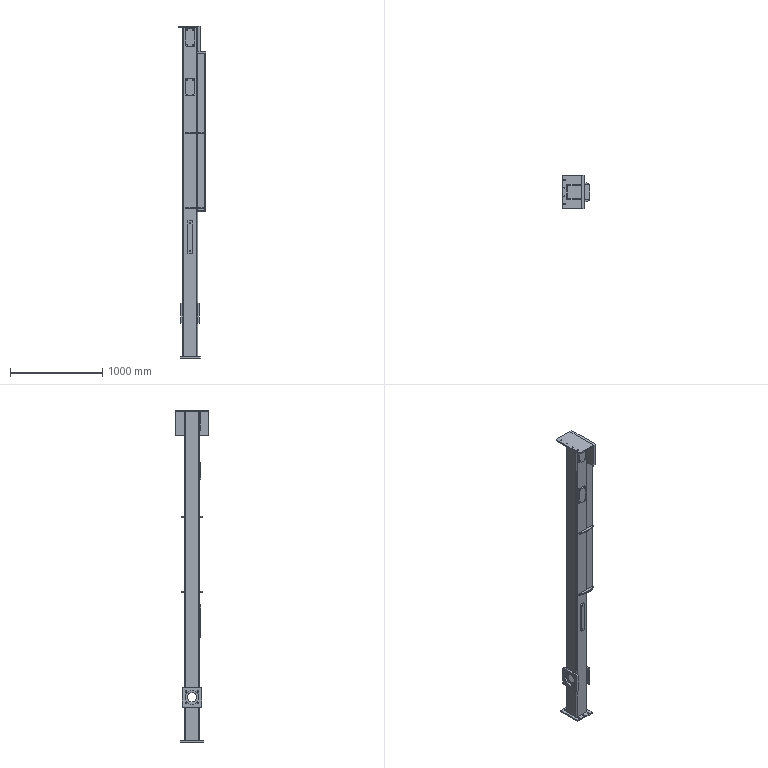Part | SolidWorks | features ICE 40, MoveCopyBody 14, HoleWzd 8, MirrorSolid 7, MoveFace 7, LPattern 6, Gusset 4, CombineBodies 2, Fillet 2, Split 2, Cut 1, DelFace 1, WeldMemberFeat 1, WeldmentFeature 1 | 20 solids | 246 faces | box 300 x 360 x 3598 mm | volume 23112152 mm3 | plane 120 | cylinder 114 | cone 8 | spline 4 | commonest cylinder face diameters 10.2 x24 20 x22 15.5 x16 18 x12 6.8 x8 9 x8